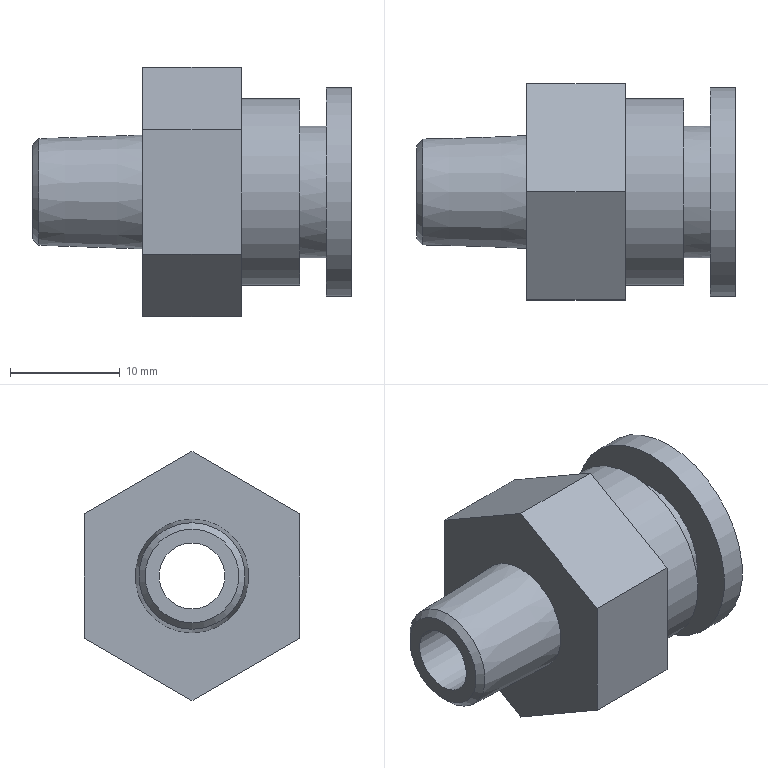Part | STEP file | solid 118 | 1 solid | 18 faces | box 29 x 19.63 x 22.667 mm | volume 5092 mm3 | plane 12 | cylinder 4 | cone 2 | commonest cylinder face diameters 6 x1 12 x1 17 x1 19 x1